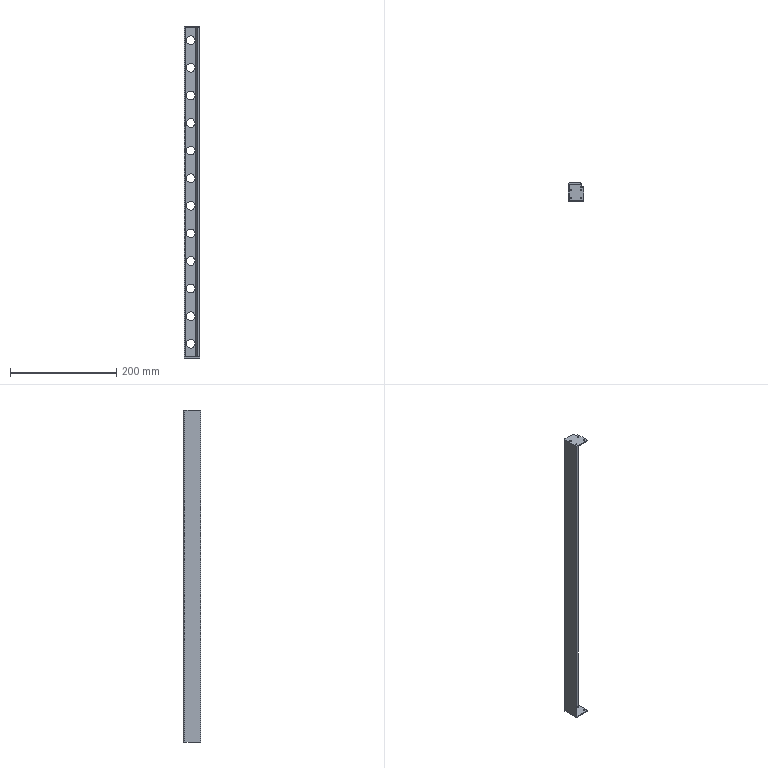Part | STEP file | Storage display board | 1 solid | 60 faces | box 30 x 33 x 626 mm | volume 79983 mm3 | cylinder 46 | plane 14 | commonest cylinder face diameters 16.5 x24 2.5 x16 2 x3 6 x3